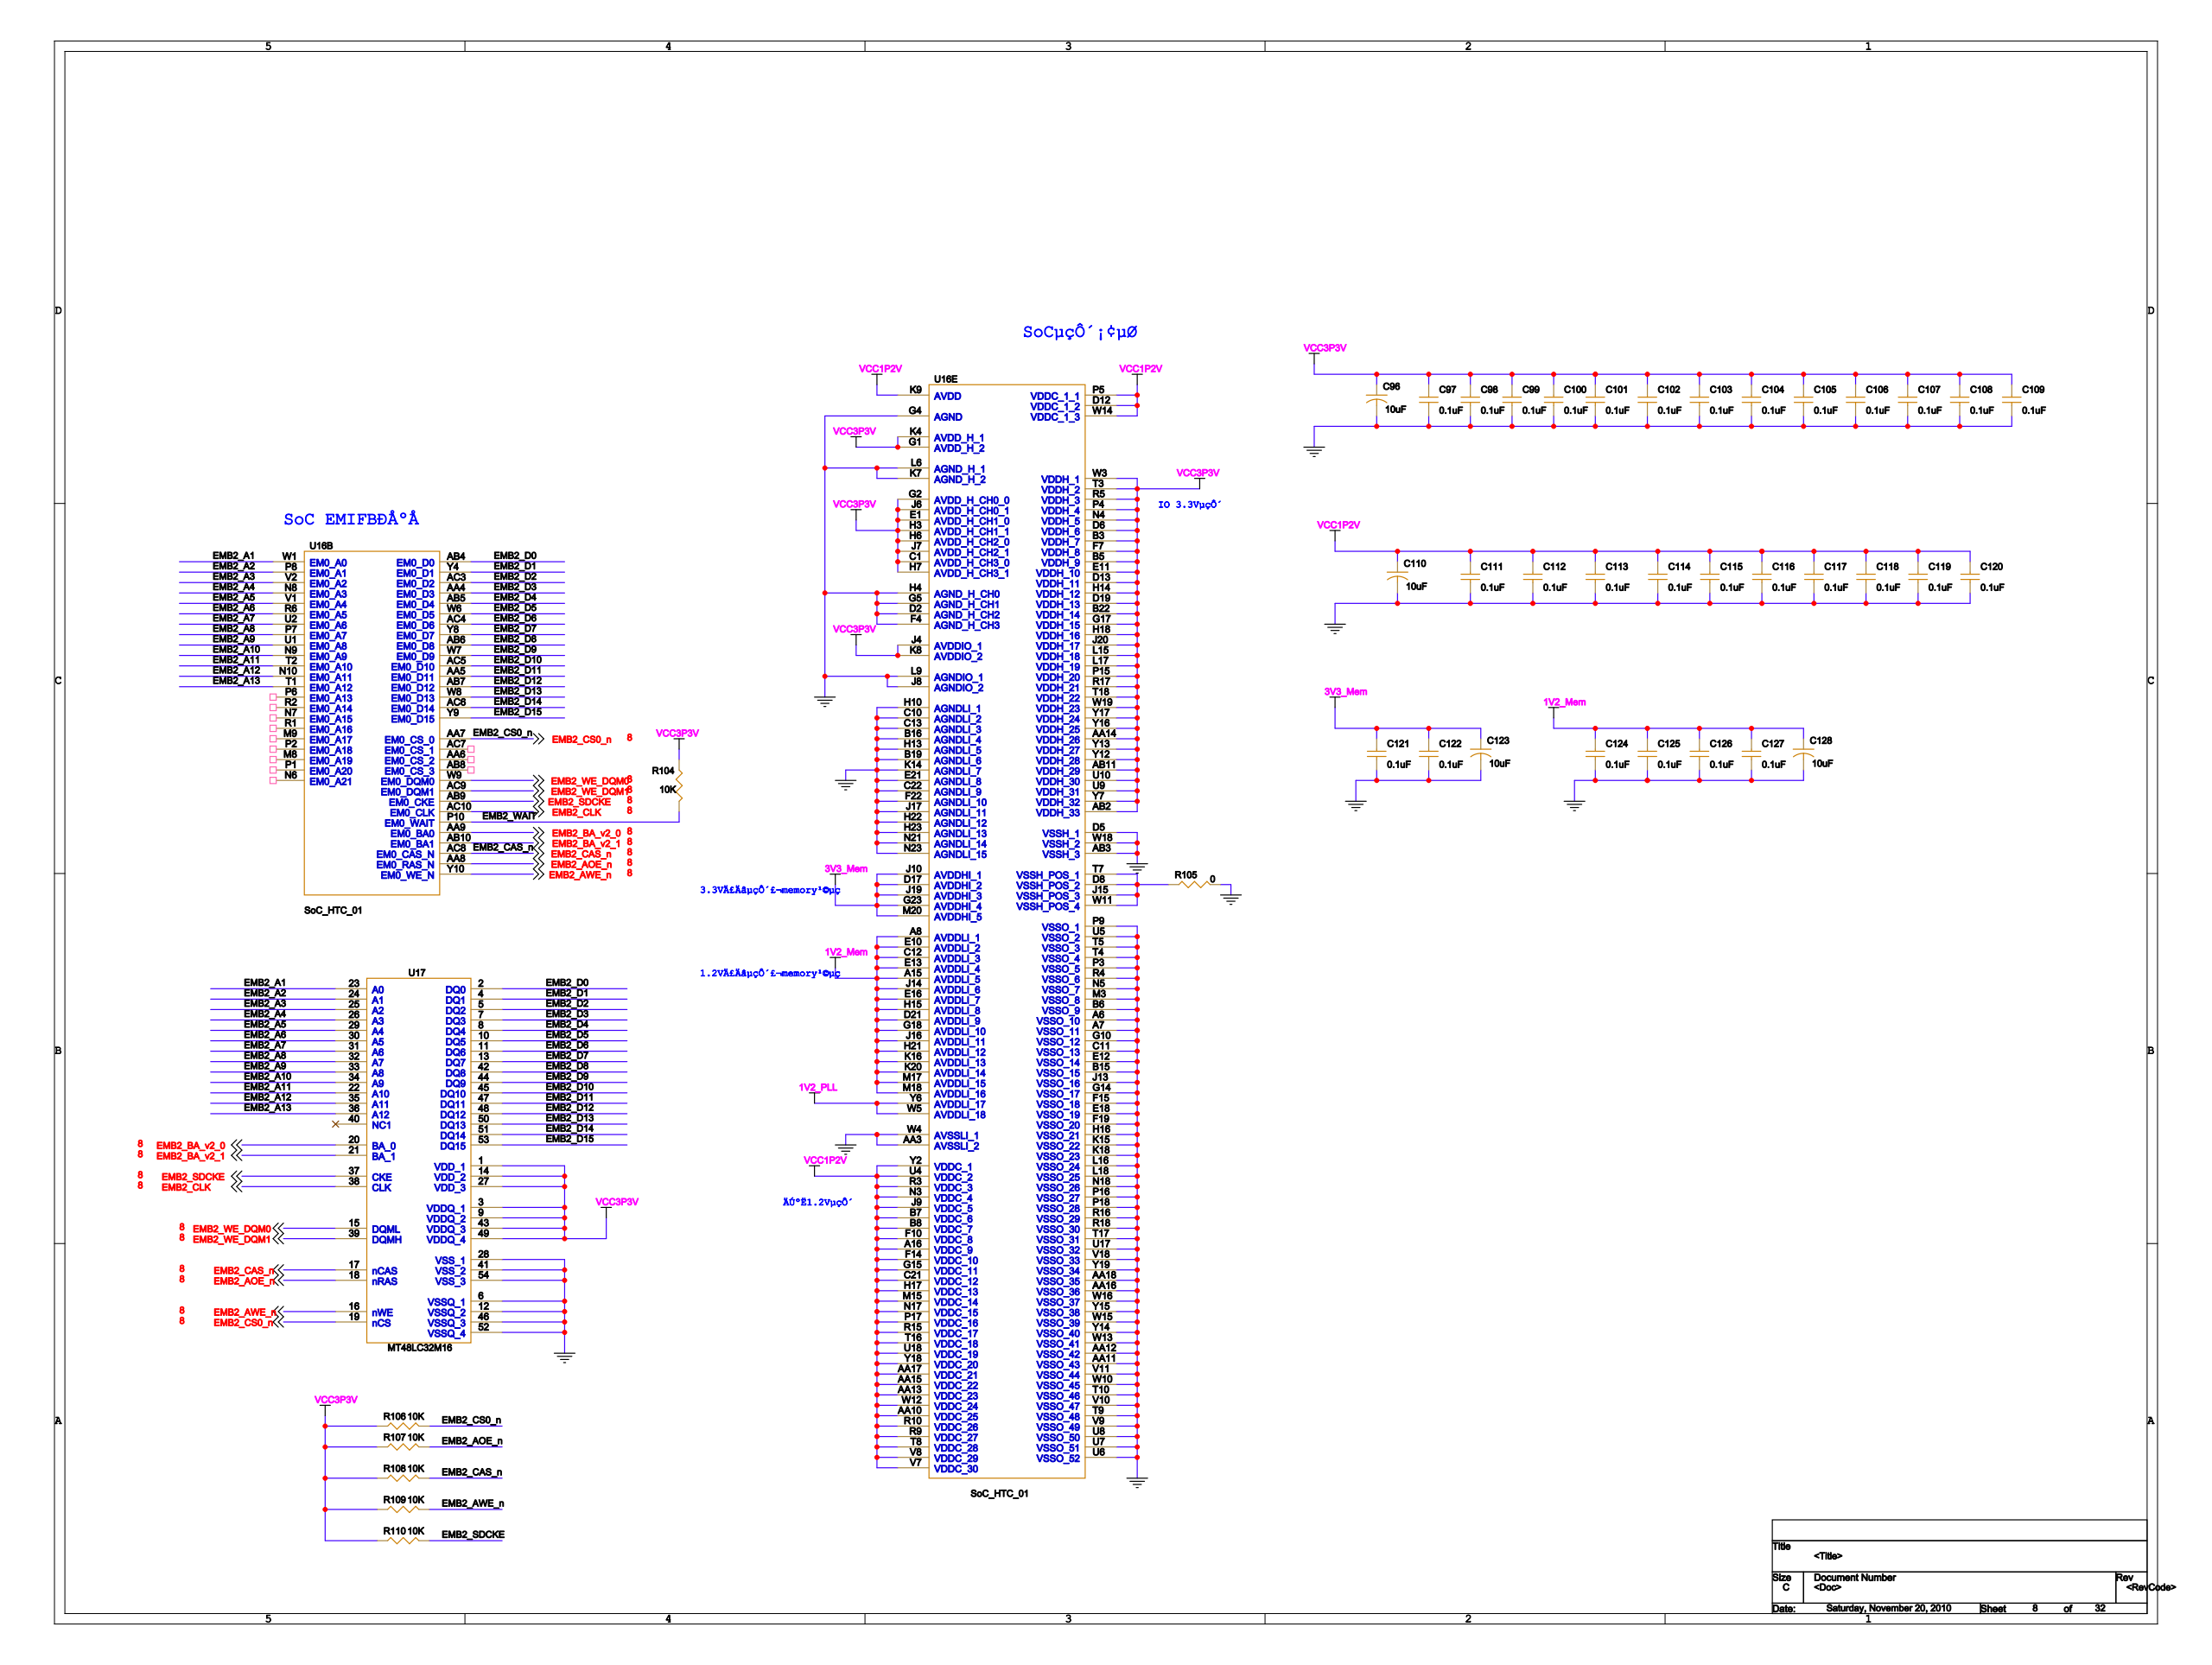Circuit board | Cadence Allegro | 1001 parts | 1318 nets | one sheet of the schematic
Parts on this sheet (reference | value | footprint):
C96 | 10uF | C3216
C97 | 0.1uF | C0402
C98 | 0.1uF | C0402
C99 | 0.1uF | C0402
C100 | 0.1uF | C0402
C101 | 0.1uF | C0402
C102 | 0.1uF | C0402
C103 | 0.1uF | C0402
C104 | 0.1uF | C0402
C105 | 0.1uF | C0402
C106 | 0.1uF | C0402
C107 | 0.1uF | C0402
C108 | 0.1uF | C0402
C109 | 0.1uF | C0402
C110 | 10uF | C3216
C111 | 0.1uF | C0402
C112 | 0.1uF | C0402
C113 | 0.1uF | C0402
C114 | 0.1uF | C0402
C115 | 0.1uF | C0402
C116 | 0.1uF | C0402
C117 | 0.1uF | C0402
C118 | 0.1uF | C0402
C119 | 0.1uF | C0402
C120 | 0.1uF | C0402
C121 | 0.1uF | C0402
C122 | 0.1uF | C0402
C123 | 10uF | C3216
C124 | 0.1uF | C0402
C125 | 0.1uF | C0402
C126 | 0.1uF | C0402
C127 | 0.1uF | C0402
C128 | 10uF | C3216
R104 | 10K | 0603
R105 | 0 | 0603
R106 | 10K | 0603
R107 | 10K | 0603
R108 | 10K | 0603
R109 | 10K | 0603
R110 | 10K | 0603
U1 | SoC_HTC_01 | L529_XIN
U2 | MT48LC32M16 | TSOP54
U4 | MAX3243 | TSSOP-28
U6 | MT48LC16M16 | TSOP54
U7 | MT48LC16M16 | TSOP54
U8 | DP83848C | DP83848C_48LQFP
U10 | SoC_HTC_01 | L529_XIN
U16 | SoC_HTC_01 | L529_XIN
U17 | MT48LC32M16 | TSOP54
Nets of these parts (net: part-pin ...):
GND: C96-2 C97-2 C98-2 C99-2 C100-2 C101-2 C102-2 C103-2 C104-2 C105-2 C106-2 C107-2 C108-2 C109-2 C110-2 C111-2 C112-2 C113-2 C114-2 C115-2 C116-2 C117-2 C118-2 C119-2 C120-2 C121-2 C122-2 C123-2 C124-2 C125-2 C126-2 C127-2 C128-2 R105-2 U1-A6 U1-A7 U1-AA3 U1-AA11 U1-AA12 U1-AA16 U1-AA18 U1-AB3 U1-B6 U1-B15 U1-B16 U1-B19 U1-C10 U1-C11 U1-C13 U1-C22 U1-D2 U1-D5 U1-E12 U1-E18 U1-E21 U1-F4 U1-F15 U1-F19 U1-F22 U1-G4 U1-G5 U1-G10 U1-G14 U1-H4 U1-H10 U1-H13 U1-H16 U1-H22 U1-H23 U1-J8 U1-J13 U1-J17 U1-K7 U1-K14 U1-K15 U1-K18 U1-L6 U1-L9 U1-L16 U1-L18 U1-M3 U1-N5 U1-N18 U1-N21 U1-N23 U1-P3 U1-P9 U1-P16 U1-P18 U1-R4 U1-R16 U1-R18 U1-T4 U1-T5 U1-T9 U1-T10 U1-T17 U1-U5 U1-U6 U1-U7 U1-U8 U1-U17 U1-V9 U1-V10 U1-V11 U1-V18 U1-W4 U1-W10 U1-W13 U1-W15 U1-W16 U1-W18 U1-Y14 U1-Y15 U1-Y19 U2-6 U2-12 U2-28 U2-41 U2-46 U2-52 U2-54 U4-23 U4-25 U6-6 U6-12 U6-28 U6-41 U6-46 U6-52 U6-54 U7-6 U7-12 U7-28 U7-41 U7-46 U7-52 U7-54 U8-15 U8-19 U8-35 U8-36 U8-47 U10-A6 U10-A7 U10-AA3 U10-AA11 U10-AA12 U10-AA16 U10-AA18 U10-AB3 U10-B6 U10-B15 U10-B16 U10-B19 U10-C10 U10-C11 U10-C13 U10-C22 U10-D2 U10-D5 U10-E12 U10-E18 U10-E21 U10-F4 U10-F15 U10-F19 U10-F22 U10-G4 U10-G5 U10-G10 U10-G14 U10-H4 U10-H10 U10-H13 U10-H16 U10-H22 U10-H23 U10-J8 U10-J13 U10-J17 U10-K7 U10-K14 U10-K15 U10-K18 U10-L6 U10-L9 U10-L16 U10-L18 U10-M3 U10-N5 U10-N18 U10-N21 U10-N23 U10-P3 U10-P9 U10-P16 U10-P18 U10-R4 U10-R16 U10-R18 U10-T4 U10-T5 U10-T9 U10-T10 U10-T17 U10-U5 U10-U6 U10-U7 U10-U8 U10-U17 U10-V9 U10-V10 U10-V11 U10-V18 U10-W4 U10-W10 U10-W13 U10-W15 U10-W16 U10-W18 U10-Y14 U10-Y15 U10-Y19 U16-A6 U16-A7 U16-AA3 U16-AA11 U16-AA12 U16-AA16 U16-AA18 U16-AB3 U16-B6 U16-B15 U16-B16 U16-B19 U16-C10 U16-C11 U16-C13 U16-C22 U16-D2 U16-D5 U16-E12 U16-E18 U16-E21 U16-F4 U16-F15 U16-F19 U16-F22 U16-G4 U16-G5 U16-G10 U16-G14 U16-H4 U16-H10 U16-H13 U16-H16 U16-H22 U16-H23 U16-J8 U16-J13 U16-J17 U16-K7 U16-K14 U16-K15 U16-K18 U16-L6 U16-L9 U16-L16 U16-L18 U16-M3 U16-N5 U16-N18 U16-N21 U16-N23 U16-P3 U16-P9 U16-P16 U16-P18 U16-R4 U16-R16 U16-R18 U16-T4 U16-T5 U16-T9 U16-T10 U16-T17 U16-U5 U16-U6 U16-U7 U16-U8 U16-U17 U16-V9 U16-V10 U16-V11 U16-V18 U16-W4 U16-W10 U16-W13 U16-W15 U16-W16 U16-W18 U16-Y14 U16-Y15 U16-Y19 U17-6 U17-12 U17-28 U17-41 U17-46 U17-52 U17-54
VCC3P3V: C96-1 C97-1 C98-1 C99-1 C100-1 C101-1 C102-1 C103-1 C104-1 C105-1 C106-1 C107-1 C108-1 C109-1 R104-2 R106-1 R107-1 R108-1 R109-1 R110-1 U1-AA14 U1-AB2 U1-AB11 U1-B3 U1-B5 U1-B22 U1-C1 U1-D6 U1-D13 U1-D19 U1-E1 U1-E11 U1-F7 U1-G1 U1-G2 U1-G17 U1-H3 U1-H6 U1-H7 U1-H14 U1-H18 U1-J4 U1-J6 U1-J7 U1-J20 U1-K4 U1-K8 U1-L15 U1-L17 U1-N4 U1-P4 U1-P15 U1-R5 U1-R17 U1-T3 U1-T18 U1-U9 U1-U10 U1-W3 U1-W19 U1-Y7 U1-Y12 U1-Y13 U1-Y16 U1-Y17 U2-1 U2-3 U2-9 U2-14 U2-27 U2-43 U2-49 U4-22 U4-26 U6-1 U6-3 U6-9 U6-14 U6-27 U6-43 U6-49 U7-1 U7-3 U7-9 U7-14 U7-27 U7-43 U7-49 U8-22 U8-32 U8-48 U10-AA14 U10-AB2 U10-AB11 U10-B3 U10-B5 U10-B22 U10-C1 U10-D6 U10-D13 U10-D19 U10-E1 U10-E11 U10-F7 U10-G1 U10-G2 U10-G17 U10-H3 U10-H6 U10-H7 U10-H14 U10-H18 U10-J4 U10-J6 U10-J7 U10-J20 U10-K4 U10-K8 U10-L15 U10-L17 U10-N4 U10-P4 U10-P15 U10-R5 U10-R17 U10-T3 U10-T18 U10-U9 U10-U10 U10-W3 U10-W19 U10-Y7 U10-Y12 U10-Y13 U10-Y16 U10-Y17 U16-AA14 U16-AB2 U16-AB11 U16-B3 U16-B5 U16-B22 U16-C1 U16-D6 U16-D13 U16-D19 U16-E1 U16-E11 U16-F7 U16-G1 U16-G2 U16-G17 U16-H3 U16-H6 U16-H7 U16-H14 U16-H18 U16-J4 U16-J6 U16-J7 U16-J20 U16-K4 U16-K8 U16-L15 U16-L17 U16-N4 U16-P4 U16-P15 U16-R5 U16-R17 U16-T3 U16-T18 U16-U9 U16-U10 U16-W3 U16-W19 U16-Y7 U16-Y12 U16-Y13 U16-Y16 U16-Y17 U17-1 U17-3 U17-9 U17-14 U17-27 U17-43 U17-49
VCC1P2V: C110-1 C111-1 C112-1 C113-1 C114-1 C115-1 C116-1 C117-1 C118-1 C119-1 C120-1 U1-A16 U1-AA10 U1-AA13 U1-AA15 U1-AA17 U1-B7 U1-B8 U1-C21 U1-D12 U1-F10 U1-F14 U1-G15 U1-H17 U1-J9 U1-K9 U1-M15 U1-N3 U1-N17 U1-P5 U1-P17 U1-R3 U1-R9 U1-R10 U1-R15 U1-T8 U1-T16 U1-U4 U1-U18 U1-V7 U1-V8 U1-W12 U1-W14 U1-Y2 U1-Y18 U10-A16 U10-AA10 U10-AA13 U10-AA15 U10-AA17 U10-B7 U10-B8 U10-C21 U10-D12 U10-F10 U10-F14 U10-G15 U10-H17 U10-J9 U10-K9 U10-M15 U10-N3 U10-N17 U10-P5 U10-P17 U10-R3 U10-R9 U10-R10 U10-R15 U10-T8 U10-T16 U10-U4 U10-U18 U10-V7 U10-V8 U10-W12 U10-W14 U10-Y2 U10-Y18 U16-A16 U16-AA10 U16-AA13 U16-AA15 U16-AA17 U16-B7 U16-B8 U16-C21 U16-D12 U16-F10 U16-F14 U16-G15 U16-H17 U16-J9 U16-K9 U16-M15 U16-N3 U16-N17 U16-P5 U16-P17 U16-R3 U16-R9 U16-R10 U16-R15 U16-T8 U16-T16 U16-U4 U16-U18 U16-V7 U16-V8 U16-W12 U16-W14 U16-Y2 U16-Y18
3V3_MEM: C121-1 C122-1 C123-1 U1-D17 U1-G23 U1-J10 U1-J19 U1-M20 U10-D17 U10-G23 U10-J10 U10-J19 U10-M20 U16-D17 U16-G23 U16-J10 U16-J19 U16-M20
1V2_MEM: C124-1 C125-1 C126-1 C127-1 C128-1 U1-A8 U1-A15 U1-C12 U1-D21 U1-E10 U1-E13 U1-E16 U1-G18 U1-H15 U1-H21 U1-J14 U1-J16 U1-K16 U1-K20 U1-M17 U1-M18 U10-A8 U10-A15 U10-C12 U10-D21 U10-E10 U10-E13 U10-E16 U10-G18 U10-H15 U10-H21 U10-J14 U10-J16 U10-K16 U10-K20 U10-M17 U10-M18 U16-A8 U16-A15 U16-C12 U16-D21 U16-E10 U16-E13 U16-E16 U16-G18 U16-H15 U16-H21 U16-J14 U16-J16 U16-K16 U16-K20 U16-M17 U16-M18
1V2_PLL: U1-W5 U1-Y6 U10-W5 U10-Y6 U16-W5 U16-Y6
EMB2_A1: U16-W1 U17-23
EMB2_A2: U16-P8 U17-24
EMB2_A11: U16-T2 U17-22
EMB2_A12: U16-N10 U17-35
EMB2_A13: U16-T1 U17-36
EMB2_A3: U16-V2 U17-25
EMB2_A4: U16-N8 U17-26
EMB2_A5: U16-V1 U17-29
EMB2_A6: U16-R6 U17-30
EMB2_A7: U16-U2 U17-31
EMB2_A8: U16-P7 U17-32
EMB2_A9: U16-U1 U17-33
EMB2_A10: U16-N9 U17-34
EMB2_CAS_N: R108-2 U16-AC8 U17-17
EMB2_SDCKE: R110-2 U16-AB9 U17-37
EMB2_CLK: U16-AC10 U17-38
EMB2_CS0_N: R106-2 U16-AA7 U17-19
EMB2_D0: U16-AB4 U17-2
EMB2_D1: U16-Y4 U17-4
EMB2_D10: U16-AC5 U17-45
EMB2_D11: U16-AA5 U17-47
EMB2_D12: U16-AB7 U17-48
EMB2_D13: U16-W8 U17-50
EMB2_D14: U16-AC6 U17-51
EMB2_D15: U16-Y9 U17-53
EMB2_D2: U16-AC3 U17-5
EMB2_D3: U16-AA4 U17-7
EMB2_D4: U16-AB5 U17-8
EMB2_D5: U16-W6 U17-10
EMB2_D6: U16-AC4 U17-11
EMB2_D7: U16-Y8 U17-13
EMB2_D8: U16-AB6 U17-42
EMB2_D9: U16-W7 U17-44
EMB2_WE_DQM0: U16-W9 U17-15
EMB2_WE_DQM1: U16-AC9 U17-39
EMB2_AOE_N: R107-2 U16-AA8 U17-18
EMB2_WAIT: R104-1 U16-P10
EMB2_AWE_N: R109-2 U16-Y10 U17-16
N17400171: R105-1 U16-D8 U16-J15 U16-T7 U16-W11